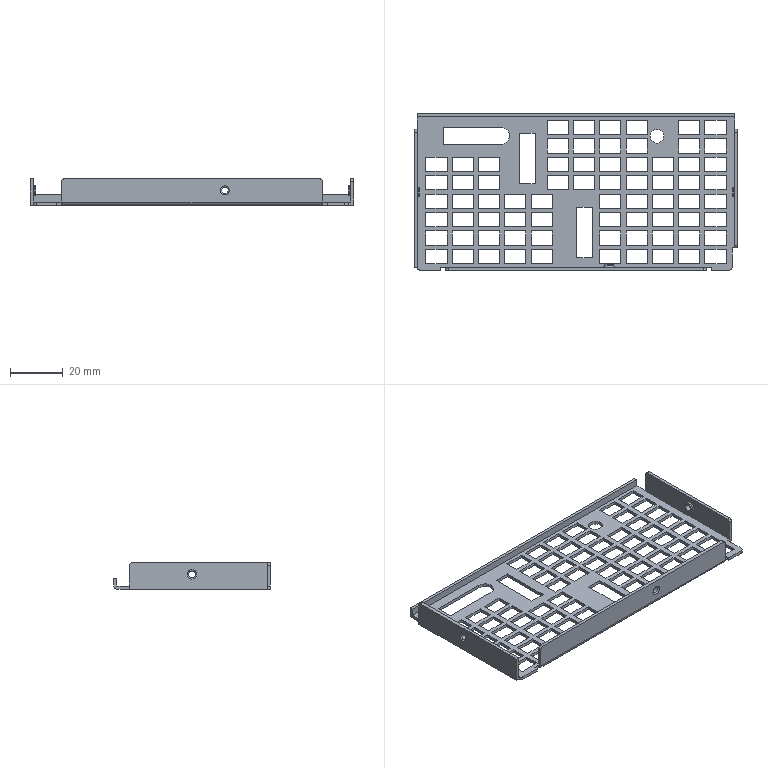Part | NX | features BREP 1 | 1 solid | 354 faces | box 123 x 59.5 x 10 mm | volume 6917 mm3 | plane 331 | cylinder 17 | torus 6 | commonest cylinder face diameters 2 x5 2.4 x4 2.5 x3 3.7 x3 5.2 x1 6.6 x1